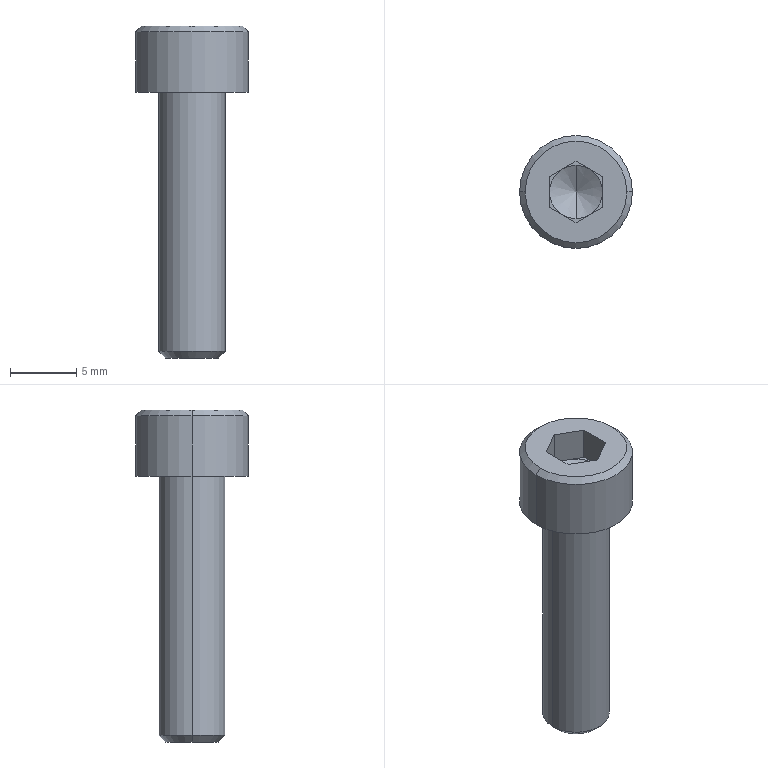Part | NX | features BREP 1 | 1 solid | 25 faces | box 8.5 x 8.5 x 25 mm | volume 632.849 mm3 | plane 15 | cone 6 | cylinder 4 | commonest cylinder face diameters 5 x2 8.5 x2
STEP:
#1=CARTESIAN_POINT('',(0.,-2.,2.5));
#2=VERTEX_POINT('',#1);
#3=CARTESIAN_POINT('',(0.,0.,1.345));
#4=VERTEX_POINT('',#3);
#5=CARTESIAN_POINT('',(0.,0.,1.345));
#6=DIRECTION('',(0.,-0.866,0.5));
#7=VECTOR('',#6,1000.);
#8=LINE('',#5,#7);
#9=EDGE_CURVE('',#2,#4,#8,.F.);
#10=ORIENTED_EDGE('',*,*,#9,.T.);
#11=CARTESIAN_POINT('',(0.,2.,2.5));
#12=VERTEX_POINT('',#11);
#13=CARTESIAN_POINT('',(0.,0.,1.345));
#14=DIRECTION('',(0.,0.866,0.5));
#15=VECTOR('',#14,1000.);
#16=LINE('',#13,#15);
#17=EDGE_CURVE('',#12,#4,#16,.F.);
#18=ORIENTED_EDGE('',*,*,#17,.F.);
#19=CARTESIAN_POINT('',(-1.,1.732,2.5));
#20=VERTEX_POINT('',#19);
#21=CARTESIAN_POINT('',(0.,0.,2.5));
#22=DIRECTION('',(0.,0.,1.));
#23=DIRECTION('',(0.,-1.,0.));
#24=AXIS2_PLACEMENT_3D('',#21,#22,#23);
#25=CIRCLE('',#24,2.);
#26=EDGE_CURVE('',#12,#20,#25,.T.);
#27=ORIENTED_EDGE('',*,*,#26,.T.);
#28=CARTESIAN_POINT('',(-2.,0.,2.5));
#29=VERTEX_POINT('',#28);
#30=CARTESIAN_POINT('',(0.,0.,2.5));
#31=DIRECTION('',(0.,0.,1.));
#32=DIRECTION('',(0.,-1.,0.));
#33=AXIS2_PLACEMENT_3D('',#30,#31,#32);
#34=CIRCLE('',#33,2.);
#35=EDGE_CURVE('',#20,#29,#34,.T.);
#36=ORIENTED_EDGE('',*,*,#35,.T.);
#37=CARTESIAN_POINT('',(-1.,-1.732,2.5));
#38=VERTEX_POINT('',#37);
#39=CARTESIAN_POINT('',(0.,0.,2.5));
#40=DIRECTION('',(0.,0.,1.));
#41=DIRECTION('',(0.,-1.,0.));
#42=AXIS2_PLACEMENT_3D('',#39,#40,#41);
#43=CIRCLE('',#42,2.);
#44=EDGE_CURVE('',#29,#38,#43,.T.);
#45=ORIENTED_EDGE('',*,*,#44,.T.);
#46=CARTESIAN_POINT('',(0.,0.,2.5));
#47=DIRECTION('',(0.,0.,1.));
#48=DIRECTION('',(0.,-1.,0.));
#49=AXIS2_PLACEMENT_3D('',#46,#47,#48);
#50=CIRCLE('',#49,2.);
#51=EDGE_CURVE('',#38,#2,#50,.T.);
#52=ORIENTED_EDGE('',*,*,#51,.T.);
#53=EDGE_LOOP('',(#10,#18,#27,#36,#45,#52));
#54=FACE_BOUND('',#53,.T.);
#55=CARTESIAN_POINT('',(0.,0.,1001.345));
#56=DIRECTION('',(0.,0.,1.));
#57=DIRECTION('',(0.,1.,0.));
#58=AXIS2_PLACEMENT_3D('',#55,#56,#57);
#59=CONICAL_SURFACE('',#58,1732.051,1.047);
#60=ADVANCED_FACE('',(#54),#59,.F.);
#61=CARTESIAN_POINT('',(4.25,0.,0.));
#62=VERTEX_POINT('',#61);
#63=CARTESIAN_POINT('',(-4.25,0.,0.));
#64=VERTEX_POINT('',#63);
#65=CARTESIAN_POINT('',(0.,0.,0.));
#66=DIRECTION('',(0.,0.,1.));
#67=DIRECTION('',(1.,0.,0.));
#68=AXIS2_PLACEMENT_3D('',#65,#66,#67);
#69=CIRCLE('',#68,4.25);
#70=EDGE_CURVE('',#62,#64,#69,.T.);
#71=ORIENTED_EDGE('',*,*,#70,.T.);
#72=CARTESIAN_POINT('',(-4.25,0.,4.575));
#73=VERTEX_POINT('',#72);
#74=CARTESIAN_POINT('',(-4.25,0.,0.));
#75=DIRECTION('',(0.,0.,1.));
#76=VECTOR('',#75,1000.);
#77=LINE('',#74,#76);
#78=EDGE_CURVE('',#64,#73,#77,.T.);
#79=ORIENTED_EDGE('',*,*,#78,.T.);
#80=CARTESIAN_POINT('',(4.25,0.,4.575));
#81=VERTEX_POINT('',#80);
#82=CARTESIAN_POINT('',(0.,0.,4.575));
#83=DIRECTION('',(0.,0.,1.));
#84=DIRECTION('',(1.,0.,0.));
#85=AXIS2_PLACEMENT_3D('',#82,#83,#84);
#86=CIRCLE('',#85,4.25);
#87=EDGE_CURVE('',#81,#73,#86,.T.);
#88=ORIENTED_EDGE('',*,*,#87,.F.);
#89=CARTESIAN_POINT('',(4.25,0.,0.));
#90=DIRECTION('',(0.,0.,1.));
#91=VECTOR('',#90,1000.);
#92=LINE('',#89,#91);
#93=EDGE_CURVE('',#62,#81,#92,.T.);
#94=ORIENTED_EDGE('',*,*,#93,.F.);
#95=EDGE_LOOP('',(#71,#79,#88,#94));
#96=FACE_BOUND('',#95,.T.);
#97=CARTESIAN_POINT('',(0.,0.,0.));
#98=DIRECTION('',(0.,0.,1.));
#99=DIRECTION('',(-1.,0.,0.));
#100=AXIS2_PLACEMENT_3D('',#97,#98,#99);
#101=CYLINDRICAL_SURFACE('',#100,4.25);
#102=ADVANCED_FACE('',(#96),#101,.T.);
#103=CARTESIAN_POINT('',(3.825,0.,5.));
#104=VERTEX_POINT('',#103);
#105=CARTESIAN_POINT('',(-3.825,0.,5.));
#106=VERTEX_POINT('',#105);
#107=CARTESIAN_POINT('',(0.,0.,5.));
#108=DIRECTION('',(0.,0.,1.));
#109=DIRECTION('',(1.,0.,0.));
#110=AXIS2_PLACEMENT_3D('',#107,#108,#109);
#111=CIRCLE('',#110,3.825);
#112=EDGE_CURVE('',#104,#106,#111,.T.);
#113=ORIENTED_EDGE('',*,*,#112,.F.);
#114=CARTESIAN_POINT('',(4.25,0.,4.575));
#115=DIRECTION('',(0.7071,0.,-0.7071));
#116=VECTOR('',#115,1000.);
#117=LINE('',#114,#116);
#118=EDGE_CURVE('',#81,#104,#117,.F.);
#119=ORIENTED_EDGE('',*,*,#118,.F.);
#120=ORIENTED_EDGE('',*,*,#87,.T.);
#121=CARTESIAN_POINT('',(-4.25,0.,4.575));
#122=DIRECTION('',(-0.7071,0.,-0.7071));
#123=VECTOR('',#122,1000.);
#124=LINE('',#121,#123);
#125=EDGE_CURVE('',#73,#106,#124,.F.);
#126=ORIENTED_EDGE('',*,*,#125,.T.);
#127=EDGE_LOOP('',(#113,#119,#120,#126));
#128=FACE_BOUND('',#127,.T.);
#129=CARTESIAN_POINT('',(0.,0.,4.575));
#130=DIRECTION('',(0.,0.,-1.));
#131=DIRECTION('',(1.,0.,0.));
#132=AXIS2_PLACEMENT_3D('',#129,#130,#131);
#133=CONICAL_SURFACE('',#132,4.25,0.7854);
#134=ADVANCED_FACE('',(#128),#133,.T.);
#135=CARTESIAN_POINT('',(2.01,0.,-20.));
#136=VERTEX_POINT('',#135);
#137=CARTESIAN_POINT('',(-2.01,0.,-20.));
#138=VERTEX_POINT('',#137);
#139=CARTESIAN_POINT('',(0.,0.,-20.));
#140=DIRECTION('',(0.,0.,1.));
#141=DIRECTION('',(1.,0.,0.));
#142=AXIS2_PLACEMENT_3D('',#139,#140,#141);
#143=CIRCLE('',#142,2.01);
#144=EDGE_CURVE('',#136,#138,#143,.T.);
#145=ORIENTED_EDGE('',*,*,#144,.T.);
#146=CARTESIAN_POINT('',(-2.5,0.,-19.509));
#147=VERTEX_POINT('',#146);
#148=CARTESIAN_POINT('',(-2.01,0.,-20.));
#149=DIRECTION('',(-0.7071,0.,0.7071));
#150=VECTOR('',#149,1000.);
#151=LINE('',#148,#150);
#152=EDGE_CURVE('',#138,#147,#151,.T.);
#153=ORIENTED_EDGE('',*,*,#152,.T.);
#154=CARTESIAN_POINT('',(2.5,0.,-19.509));
#155=VERTEX_POINT('',#154);
#156=CARTESIAN_POINT('',(0.,0.,-19.509));
#157=DIRECTION('',(0.,0.,1.));
#158=DIRECTION('',(1.,0.,0.));
#159=AXIS2_PLACEMENT_3D('',#156,#157,#158);
#160=CIRCLE('',#159,2.5);
#161=EDGE_CURVE('',#155,#147,#160,.T.);
#162=ORIENTED_EDGE('',*,*,#161,.F.);
#163=CARTESIAN_POINT('',(2.01,0.,-20.));
#164=DIRECTION('',(0.7071,0.,0.7071));
#165=VECTOR('',#164,1000.);
#166=LINE('',#163,#165);
#167=EDGE_CURVE('',#136,#155,#166,.T.);
#168=ORIENTED_EDGE('',*,*,#167,.F.);
#169=EDGE_LOOP('',(#145,#153,#162,#168));
#170=FACE_BOUND('',#169,.T.);
#171=CARTESIAN_POINT('',(0.,0.,-20.));
#172=DIRECTION('',(0.,0.,1.));
#173=DIRECTION('',(-1.,0.,0.));
#174=AXIS2_PLACEMENT_3D('',#171,#172,#173);
#175=CONICAL_SURFACE('',#174,2.01,0.7854);
#176=ADVANCED_FACE('',(#170),#175,.T.);
#177=ORIENTED_EDGE('',*,*,#161,.T.);
#178=CARTESIAN_POINT('',(-2.5,0.,0.));
#179=VERTEX_POINT('',#178);
#180=CARTESIAN_POINT('',(-2.5,0.,-20.));
#181=DIRECTION('',(0.,0.,1.));
#182=VECTOR('',#181,1000.);
#183=LINE('',#180,#182);
#184=EDGE_CURVE('',#147,#179,#183,.T.);
#185=ORIENTED_EDGE('',*,*,#184,.T.);
#186=CARTESIAN_POINT('',(2.5,0.,0.));
#187=VERTEX_POINT('',#186);
#188=CARTESIAN_POINT('',(0.,0.,0.));
#189=DIRECTION('',(0.,0.,1.));
#190=DIRECTION('',(1.,0.,0.));
#191=AXIS2_PLACEMENT_3D('',#188,#189,#190);
#192=CIRCLE('',#191,2.5);
#193=EDGE_CURVE('',#187,#179,#192,.T.);
#194=ORIENTED_EDGE('',*,*,#193,.F.);
#195=CARTESIAN_POINT('',(2.5,0.,-20.));
#196=DIRECTION('',(0.,0.,1.));
#197=VECTOR('',#196,1000.);
#198=LINE('',#195,#197);
#199=EDGE_CURVE('',#155,#187,#198,.T.);
#200=ORIENTED_EDGE('',*,*,#199,.F.);
#201=EDGE_LOOP('',(#177,#185,#194,#200));
#202=FACE_BOUND('',#201,.T.);
#203=CARTESIAN_POINT('',(0.,0.,-20.));
#204=DIRECTION('',(0.,0.,1.));
#205=DIRECTION('',(-1.,0.,0.));
#206=AXIS2_PLACEMENT_3D('',#203,#204,#205);
#207=CYLINDRICAL_SURFACE('',#206,2.5);
#208=ADVANCED_FACE('',(#202),#207,.T.);
#209=CARTESIAN_POINT('',(1.,-1.732,2.5));
#210=VERTEX_POINT('',#209);
#211=CARTESIAN_POINT('',(2.,0.,2.5));
#212=VERTEX_POINT('',#211);
#213=CARTESIAN_POINT('',(0.,0.,2.5));
#214=DIRECTION('',(0.,0.,1.));
#215=DIRECTION('',(0.,-1.,0.));
#216=AXIS2_PLACEMENT_3D('',#213,#214,#215);
#217=CIRCLE('',#216,2.);
#218=EDGE_CURVE('',#210,#212,#217,.T.);
#219=ORIENTED_EDGE('',*,*,#218,.F.);
#220=CARTESIAN_POINT('',(2.,-1.155,2.5));
#221=VERTEX_POINT('',#220);
#222=CARTESIAN_POINT('',(0.,-2.309,2.5));
#223=DIRECTION('',(0.866,0.5,0.));
#224=VECTOR('',#223,1000.);
#225=LINE('',#222,#224);
#226=EDGE_CURVE('',#210,#221,#225,.T.);
#227=ORIENTED_EDGE('',*,*,#226,.T.);
#228=CARTESIAN_POINT('',(2.,-1.155,2.5));
#229=DIRECTION('',(0.,1.,0.));
#230=VECTOR('',#229,1000.);
#231=LINE('',#228,#230);
#232=EDGE_CURVE('',#221,#212,#231,.T.);
#233=ORIENTED_EDGE('',*,*,#232,.T.);
#234=EDGE_LOOP('',(#219,#227,#233));
#235=FACE_BOUND('',#234,.T.);
#236=CARTESIAN_POINT('',(0.,0.,2.5));
#237=DIRECTION('',(0.,0.,1.));
#238=DIRECTION('',(-1.,0.,0.));
#239=AXIS2_PLACEMENT_3D('',#236,#237,#238);
#240=PLANE('',#239);
#241=ADVANCED_FACE('',(#235),#240,.T.);
#242=CARTESIAN_POINT('',(1.,1.732,2.5));
#243=VERTEX_POINT('',#242);
#244=CARTESIAN_POINT('',(0.,0.,2.5));
#245=DIRECTION('',(0.,0.,1.));
#246=DIRECTION('',(0.,-1.,0.));
#247=AXIS2_PLACEMENT_3D('',#244,#245,#246);
#248=CIRCLE('',#247,2.);
#249=EDGE_CURVE('',#212,#243,#248,.T.);
#250=ORIENTED_EDGE('',*,*,#249,.F.);
#251=CARTESIAN_POINT('',(2.,1.155,2.5));
#252=VERTEX_POINT('',#251);
#253=CARTESIAN_POINT('',(2.,-1.155,2.5));
#254=DIRECTION('',(0.,1.,0.));
#255=VECTOR('',#254,1000.);
#256=LINE('',#253,#255);
#257=EDGE_CURVE('',#212,#252,#256,.T.);
#258=ORIENTED_EDGE('',*,*,#257,.T.);
#259=CARTESIAN_POINT('',(2.,1.155,2.5));
#260=DIRECTION('',(-0.866,0.5,0.));
#261=VECTOR('',#260,1000.);
#262=LINE('',#259,#261);
#263=EDGE_CURVE('',#252,#243,#262,.T.);
#264=ORIENTED_EDGE('',*,*,#263,.T.);
#265=EDGE_LOOP('',(#250,#258,#264));
#266=FACE_BOUND('',#265,.T.);
#267=CARTESIAN_POINT('',(0.,0.,2.5));
#268=DIRECTION('',(0.,0.,1.));
#269=DIRECTION('',(-1.,0.,0.));
#270=AXIS2_PLACEMENT_3D('',#267,#268,#269);
#271=PLANE('',#270);
#272=ADVANCED_FACE('',(#266),#271,.T.);
#273=CARTESIAN_POINT('',(0.,0.,2.5));
#274=DIRECTION('',(0.,0.,1.));
#275=DIRECTION('',(0.,-1.,0.));
#276=AXIS2_PLACEMENT_3D('',#273,#274,#275);
#277=CIRCLE('',#276,2.);
#278=EDGE_CURVE('',#243,#12,#277,.T.);
#279=ORIENTED_EDGE('',*,*,#278,.F.);
#280=CARTESIAN_POINT('',(0.,2.309,2.5));
#281=VERTEX_POINT('',#280);
#282=CARTESIAN_POINT('',(2.,1.155,2.5));
#283=DIRECTION('',(-0.866,0.5,0.));
#284=VECTOR('',#283,1000.);
#285=LINE('',#282,#284);
#286=EDGE_CURVE('',#243,#281,#285,.T.);
#287=ORIENTED_EDGE('',*,*,#286,.T.);
#288=CARTESIAN_POINT('',(0.,2.309,2.5));
#289=DIRECTION('',(-0.866,-0.5,0.));
#290=VECTOR('',#289,1000.);
#291=LINE('',#288,#290);
#292=EDGE_CURVE('',#281,#20,#291,.T.);
#293=ORIENTED_EDGE('',*,*,#292,.T.);
#294=ORIENTED_EDGE('',*,*,#26,.F.);
#295=EDGE_LOOP('',(#279,#287,#293,#294));
#296=FACE_BOUND('',#295,.T.);
#297=CARTESIAN_POINT('',(0.,0.,2.5));
#298=DIRECTION('',(0.,0.,1.));
#299=DIRECTION('',(-1.,0.,0.));
#300=AXIS2_PLACEMENT_3D('',#297,#298,#299);
#301=PLANE('',#300);
#302=ADVANCED_FACE('',(#296),#301,.T.);
#303=ORIENTED_EDGE('',*,*,#35,.F.);
#304=CARTESIAN_POINT('',(-2.,1.155,2.5));
#305=VERTEX_POINT('',#304);
#306=CARTESIAN_POINT('',(0.,2.309,2.5));
#307=DIRECTION('',(-0.866,-0.5,0.));
#308=VECTOR('',#307,1000.);
#309=LINE('',#306,#308);
#310=EDGE_CURVE('',#20,#305,#309,.T.);
#311=ORIENTED_EDGE('',*,*,#310,.T.);
#312=CARTESIAN_POINT('',(-2.,1.155,2.5));
#313=DIRECTION('',(0.,-1.,0.));
#314=VECTOR('',#313,1000.);
#315=LINE('',#312,#314);
#316=EDGE_CURVE('',#305,#29,#315,.T.);
#317=ORIENTED_EDGE('',*,*,#316,.T.);
#318=EDGE_LOOP('',(#303,#311,#317));
#319=FACE_BOUND('',#318,.T.);
#320=CARTESIAN_POINT('',(0.,0.,2.5));
#321=DIRECTION('',(0.,0.,1.));
#322=DIRECTION('',(-1.,0.,0.));
#323=AXIS2_PLACEMENT_3D('',#320,#321,#322);
#324=PLANE('',#323);
#325=ADVANCED_FACE('',(#319),#324,.T.);
#326=ORIENTED_EDGE('',*,*,#44,.F.);
#327=CARTESIAN_POINT('',(-2.,-1.155,2.5));
#328=VERTEX_POINT('',#327);
#329=CARTESIAN_POINT('',(-2.,1.155,2.5));
#330=DIRECTION('',(0.,-1.,0.));
#331=VECTOR('',#330,1000.);
#332=LINE('',#329,#331);
#333=EDGE_CURVE('',#29,#328,#332,.T.);
#334=ORIENTED_EDGE('',*,*,#333,.T.);
#335=CARTESIAN_POINT('',(-2.,-1.155,2.5));
#336=DIRECTION('',(0.866,-0.5,0.));
#337=VECTOR('',#336,1000.);
#338=LINE('',#335,#337);
#339=EDGE_CURVE('',#328,#38,#338,.T.);
#340=ORIENTED_EDGE('',*,*,#339,.T.);
#341=EDGE_LOOP('',(#326,#334,#340));
#342=FACE_BOUND('',#341,.T.);
#343=CARTESIAN_POINT('',(0.,0.,2.5));
#344=DIRECTION('',(0.,0.,1.));
#345=DIRECTION('',(-1.,0.,0.));
#346=AXIS2_PLACEMENT_3D('',#343,#344,#345);
#347=PLANE('',#346);
#348=ADVANCED_FACE('',(#342),#347,.T.);
#349=ORIENTED_EDGE('',*,*,#184,.F.);
#350=CARTESIAN_POINT('',(0.,0.,-19.509));
#351=DIRECTION('',(0.,0.,1.));
#352=DIRECTION('',(1.,0.,0.));
#353=AXIS2_PLACEMENT_3D('',#350,#351,#352);
#354=CIRCLE('',#353,2.5);
#355=EDGE_CURVE('',#147,#155,#354,.T.);
#356=ORIENTED_EDGE('',*,*,#355,.T.);
#357=ORIENTED_EDGE('',*,*,#199,.T.);
#358=CARTESIAN_POINT('',(0.,0.,0.));
#359=DIRECTION('',(0.,0.,1.));
#360=DIRECTION('',(1.,0.,0.));
#361=AXIS2_PLACEMENT_3D('',#358,#359,#360);
#362=CIRCLE('',#361,2.5);
#363=EDGE_CURVE('',#179,#187,#362,.T.);
#364=ORIENTED_EDGE('',*,*,#363,.F.);
#365=EDGE_LOOP('',(#349,#356,#357,#364));
#366=FACE_BOUND('',#365,.T.);
#367=CARTESIAN_POINT('',(0.,0.,-20.));
#368=DIRECTION('',(0.,0.,1.));
#369=DIRECTION('',(-1.,0.,0.));
#370=AXIS2_PLACEMENT_3D('',#367,#368,#369);
#371=CYLINDRICAL_SURFACE('',#370,2.5);
#372=ADVANCED_FACE('',(#366),#371,.T.);
#373=ORIENTED_EDGE('',*,*,#152,.F.);
#374=CARTESIAN_POINT('',(0.,0.,-20.));
#375=DIRECTION('',(0.,0.,1.));
#376=DIRECTION('',(1.,0.,0.));
#377=AXIS2_PLACEMENT_3D('',#374,#375,#376);
#378=CIRCLE('',#377,2.01);
#379=EDGE_CURVE('',#138,#136,#378,.T.);
#380=ORIENTED_EDGE('',*,*,#379,.T.);
#381=ORIENTED_EDGE('',*,*,#167,.T.);
#382=ORIENTED_EDGE('',*,*,#355,.F.);
#383=EDGE_LOOP('',(#373,#380,#381,#382));
#384=FACE_BOUND('',#383,.T.);
#385=CARTESIAN_POINT('',(0.,0.,-20.));
#386=DIRECTION('',(0.,0.,1.));
#387=DIRECTION('',(-1.,0.,0.));
#388=AXIS2_PLACEMENT_3D('',#385,#386,#387);
#389=CONICAL_SURFACE('',#388,2.01,0.7854);
#390=ADVANCED_FACE('',(#384),#389,.T.);
#391=ORIENTED_EDGE('',*,*,#144,.F.);
#392=ORIENTED_EDGE('',*,*,#379,.F.);
#393=EDGE_LOOP('',(#391,#392));
#394=FACE_BOUND('',#393,.T.);
#395=CARTESIAN_POINT('',(0.,2.01,-20.));
#396=DIRECTION('',(0.,0.,1.));
#397=DIRECTION('',(-1.,0.,0.));
#398=AXIS2_PLACEMENT_3D('',#395,#396,#397);
#399=PLANE('',#398);
#400=ADVANCED_FACE('',(#394),#399,.F.);
#401=CARTESIAN_POINT('',(0.,-2.309,5.));
#402=VERTEX_POINT('',#401);
#403=CARTESIAN_POINT('',(2.,-1.155,5.));
#404=VERTEX_POINT('',#403);
#405=CARTESIAN_POINT('',(0.,-2.309,5.));
#406=DIRECTION('',(0.866,0.5,0.));
#407=VECTOR('',#406,1000.);
#408=LINE('',#405,#407);
#409=EDGE_CURVE('',#402,#404,#408,.T.);
#410=ORIENTED_EDGE('',*,*,#409,.F.);
#411=CARTESIAN_POINT('',(-2.,-1.155,5.));
#412=VERTEX_POINT('',#411);
#413=CARTESIAN_POINT('',(-2.,-1.155,5.));
#414=DIRECTION('',(0.866,-0.5,0.));
#415=VECTOR('',#414,1000.);
#416=LINE('',#413,#415);
#417=EDGE_CURVE('',#412,#402,#416,.T.);
#418=ORIENTED_EDGE('',*,*,#417,.F.);
#419=CARTESIAN_POINT('',(-2.,1.155,5.));
#420=VERTEX_POINT('',#419);
#421=CARTESIAN_POINT('',(-2.,1.155,5.));
#422=DIRECTION('',(0.,-1.,0.));
#423=VECTOR('',#422,1000.);
#424=LINE('',#421,#423);
#425=EDGE_CURVE('',#420,#412,#424,.T.);
#426=ORIENTED_EDGE('',*,*,#425,.F.);
#427=CARTESIAN_POINT('',(0.,2.309,5.));
#428=VERTEX_POINT('',#427);
#429=CARTESIAN_POINT('',(0.,2.309,5.));
#430=DIRECTION('',(-0.866,-0.5,0.));
#431=VECTOR('',#430,1000.);
#432=LINE('',#429,#431);
#433=EDGE_CURVE('',#428,#420,#432,.T.);
#434=ORIENTED_EDGE('',*,*,#433,.F.);
#435=CARTESIAN_POINT('',(2.,1.155,5.));
#436=VERTEX_POINT('',#435);
#437=CARTESIAN_POINT('',(2.,1.155,5.));
#438=DIRECTION('',(-0.866,0.5,0.));
#439=VECTOR('',#438,1000.);
#440=LINE('',#437,#439);
#441=EDGE_CURVE('',#436,#428,#440,.T.);
#442=ORIENTED_EDGE('',*,*,#441,.F.);
#443=CARTESIAN_POINT('',(2.,-1.155,5.));
#444=DIRECTION('',(0.,1.,0.));
#445=VECTOR('',#444,1000.);
#446=LINE('',#443,#445);
#447=EDGE_CURVE('',#404,#436,#446,.T.);
#448=ORIENTED_EDGE('',*,*,#447,.F.);
#449=EDGE_LOOP('',(#410,#418,#426,#434,#442,#448));
#450=FACE_BOUND('',#449,.T.);
#451=CARTESIAN_POINT('',(0.,0.,5.));
#452=DIRECTION('',(0.,0.,1.));
#453=DIRECTION('',(1.,0.,0.));
#454=AXIS2_PLACEMENT_3D('',#451,#452,#453);
#455=CIRCLE('',#454,3.825);
#456=EDGE_CURVE('',#106,#104,#455,.T.);
#457=ORIENTED_EDGE('',*,*,#456,.T.);
#458=ORIENTED_EDGE('',*,*,#112,.T.);
#459=EDGE_LOOP('',(#457,#458));
#460=FACE_BOUND('',#459,.T.);
#461=CARTESIAN_POINT('',(0.,0.,5.));
#462=DIRECTION('',(0.,0.,-1.));
#463=DIRECTION('',(1.,0.,0.));
#464=AXIS2_PLACEMENT_3D('',#461,#462,#463);
#465=PLANE('',#464);
#466=ADVANCED_FACE('',(#450,#460),#465,.F.);
#467=ORIENTED_EDGE('',*,*,#118,.T.);
#468=ORIENTED_EDGE('',*,*,#456,.F.);
#469=ORIENTED_EDGE('',*,*,#125,.F.);
#470=CARTESIAN_POINT('',(0.,0.,4.575));
#471=DIRECTION('',(0.,0.,1.));
#472=DIRECTION('',(1.,0.,0.));
#473=AXIS2_PLACEMENT_3D('',#470,#471,#472);
#474=CIRCLE('',#473,4.25);
#475=EDGE_CURVE('',#73,#81,#474,.T.);
#476=ORIENTED_EDGE('',*,*,#475,.T.);
#477=EDGE_LOOP('',(#467,#468,#469,#476));
#478=FACE_BOUND('',#477,.T.);
#479=CARTESIAN_POINT('',(0.,0.,4.575));
#480=DIRECTION('',(0.,0.,-1.));
#481=DIRECTION('',(1.,0.,0.));
#482=AXIS2_PLACEMENT_3D('',#479,#480,#481);
#483=CONICAL_SURFACE('',#482,4.25,0.7854);
#484=ADVANCED_FACE('',(#478),#483,.T.);
#485=ORIENTED_EDGE('',*,*,#78,.F.);
#486=CARTESIAN_POINT('',(0.,0.,0.));
#487=DIRECTION('',(0.,0.,1.));
#488=DIRECTION('',(1.,0.,0.));
#489=AXIS2_PLACEMENT_3D('',#486,#487,#488);
#490=CIRCLE('',#489,4.25);
#491=EDGE_CURVE('',#64,#62,#490,.T.);
#492=ORIENTED_EDGE('',*,*,#491,.T.);
#493=ORIENTED_EDGE('',*,*,#93,.T.);
#494=ORIENTED_EDGE('',*,*,#475,.F.);
#495=EDGE_LOOP('',(#485,#492,#493,#494));
#496=FACE_BOUND('',#495,.T.);
#497=CARTESIAN_POINT('',(0.,0.,0.));
#498=DIRECTION('',(0.,0.,1.));
#499=DIRECTION('',(-1.,0.,0.));
#500=AXIS2_PLACEMENT_3D('',#497,#498,#499);
#501=CYLINDRICAL_SURFACE('',#500,4.25);
#502=ADVANCED_FACE('',(#496),#501,.T.);
#503=ORIENTED_EDGE('',*,*,#193,.T.);
#504=ORIENTED_EDGE('',*,*,#363,.T.);
#505=EDGE_LOOP('',(#503,#504));
#506=FACE_BOUND('',#505,.T.);
#507=ORIENTED_EDGE('',*,*,#70,.F.);
#508=ORIENTED_EDGE('',*,*,#491,.F.);
#509=EDGE_LOOP('',(#507,#508));
#510=FACE_BOUND('',#509,.T.);
#511=CARTESIAN_POINT('',(0.,4.25,0.));
#512=DIRECTION('',(0.,0.,1.));
#513=DIRECTION('',(-1.,0.,0.));
#514=AXIS2_PLACEMENT_3D('',#511,#512,#513);
#515=PLANE('',#514);
#516=ADVANCED_FACE('',(#506,#510),#515,.F.);
#517=ORIENTED_EDGE('',*,*,#417,.T.);
#518=CARTESIAN_POINT('',(0.,-2.309,2.5));
#519=VERTEX_POINT('',#518);
#520=CARTESIAN_POINT('',(0.,-2.309,2.5));
#521=DIRECTION('',(0.,0.,1.));
#522=VECTOR('',#521,1000.);
#523=LINE('',#520,#522);
#524=EDGE_CURVE('',#519,#402,#523,.T.);
#525=ORIENTED_EDGE('',*,*,#524,.F.);
#526=CARTESIAN_POINT('',(-2.,-1.155,2.5));
#527=DIRECTION('',(0.866,-0.5,0.));
#528=VECTOR('',#527,1000.);
#529=LINE('',#526,#528);
#530=EDGE_CURVE('',#38,#519,#529,.T.);
#531=ORIENTED_EDGE('',*,*,#530,.F.);
#532=ORIENTED_EDGE('',*,*,#339,.F.);
#533=CARTESIAN_POINT('',(-2.,-1.155,2.5));
#534=DIRECTION('',(0.,0.,1.));
#535=VECTOR('',#534,1000.);
#536=LINE('',#533,#535);
#537=EDGE_CURVE('',#328,#412,#536,.T.);
#538=ORIENTED_EDGE('',*,*,#537,.T.);
#539=EDGE_LOOP('',(#517,#525,#531,#532,#538));
#540=FACE_BOUND('',#539,.T.);
#541=CARTESIAN_POINT('',(-2.,-1.155,2.5));
#542=DIRECTION('',(-0.5,-0.866,0.));
#543=DIRECTION('',(-0.866,0.5,0.));
#544=AXIS2_PLACEMENT_3D('',#541,#542,#543);
#545=PLANE('',#544);
#546=ADVANCED_FACE('',(#540),#545,.F.);
#547=ORIENTED_EDGE('',*,*,#425,.T.);
#548=ORIENTED_EDGE('',*,*,#537,.F.);
#549=ORIENTED_EDGE('',*,*,#333,.F.);
#550=ORIENTED_EDGE('',*,*,#316,.F.);
#551=CARTESIAN_POINT('',(-2.,1.155,2.5));
#552=DIRECTION('',(0.,0.,1.));
#553=VECTOR('',#552,1000.);
#554=LINE('',#551,#553);
#555=EDGE_CURVE('',#305,#420,#554,.T.);
#556=ORIENTED_EDGE('',*,*,#555,.T.);
#557=EDGE_LOOP('',(#547,#548,#549,#550,#556));
#558=FACE_BOUND('',#557,.T.);
#559=CARTESIAN_POINT('',(-2.,1.155,2.5));
#560=DIRECTION('',(-1.,0.,0.));
#561=DIRECTION('',(0.,0.,-1.));
#562=AXIS2_PLACEMENT_3D('',#559,#560,#561);
#563=PLANE('',#562);
#564=ADVANCED_FACE('',(#558),#563,.F.);
#565=ORIENTED_EDGE('',*,*,#433,.T.);
#566=ORIENTED_EDGE('',*,*,#555,.F.);
#567=ORIENTED_EDGE('',*,*,#310,.F.);
#568=ORIENTED_EDGE('',*,*,#292,.F.);
#569=CARTESIAN_POINT('',(0.,2.309,2.5));
#570=DIRECTION('',(0.,0.,1.));
#571=VECTOR('',#570,1000.);
#572=LINE('',#569,#571);
#573=EDGE_CURVE('',#281,#428,#572,.T.);
#574=ORIENTED_EDGE('',*,*,#573,.T.);
#575=EDGE_LOOP('',(#565,#566,#567,#568,#574));
#576=FACE_BOUND('',#575,.T.);
#577=CARTESIAN_POINT('',(0.,2.309,2.5));
#578=DIRECTION('',(-0.5,0.866,0.));
#579=DIRECTION('',(0.866,0.5,0.));
#580=AXIS2_PLACEMENT_3D('',#577,#578,#579);
#581=PLANE('',#580);
#582=ADVANCED_FACE('',(#576),#581,.F.);
#583=ORIENTED_EDGE('',*,*,#441,.T.);
#584=ORIENTED_EDGE('',*,*,#573,.F.);
#585=ORIENTED_EDGE('',*,*,#286,.F.);
#586=ORIENTED_EDGE('',*,*,#263,.F.);
#587=CARTESIAN_POINT('',(2.,1.155,2.5));
#588=DIRECTION('',(0.,0.,1.));
#589=VECTOR('',#588,1000.);
#590=LINE('',#587,#589);
#591=EDGE_CURVE('',#252,#436,#590,.T.);
#592=ORIENTED_EDGE('',*,*,#591,.T.);
#593=EDGE_LOOP('',(#583,#584,#585,#586,#592));
#594=FACE_BOUND('',#593,.T.);
#595=CARTESIAN_POINT('',(2.,1.155,2.5));
#596=DIRECTION('',(0.5,0.866,0.));
#597=DIRECTION('',(0.866,-0.5,0.));
#598=AXIS2_PLACEMENT_3D('',#595,#596,#597);
#599=PLANE('',#598);
#600=ADVANCED_FACE('',(#594),#599,.F.);
#601=ORIENTED_EDGE('',*,*,#447,.T.);
#602=ORIENTED_EDGE('',*,*,#591,.F.);
#603=ORIENTED_EDGE('',*,*,#257,.F.);
#604=ORIENTED_EDGE('',*,*,#232,.F.);
#605=CARTESIAN_POINT('',(2.,-1.155,2.5));
#606=DIRECTION('',(0.,0.,1.));
#607=VECTOR('',#606,1000.);
#608=LINE('',#605,#607);
#609=EDGE_CURVE('',#221,#404,#608,.T.);
#610=ORIENTED_EDGE('',*,*,#609,.T.);
#611=EDGE_LOOP('',(#601,#602,#603,#604,#610));
#612=FACE_BOUND('',#611,.T.);
#613=CARTESIAN_POINT('',(2.,-1.155,2.5));
#614=DIRECTION('',(1.,0.,0.));
#615=DIRECTION('',(0.,0.,1.));
#616=AXIS2_PLACEMENT_3D('',#613,#614,#615);
#617=PLANE('',#616);
#618=ADVANCED_FACE('',(#612),#617,.F.);
#619=ORIENTED_EDGE('',*,*,#409,.T.);
#620=ORIENTED_EDGE('',*,*,#609,.F.);
#621=ORIENTED_EDGE('',*,*,#226,.F.);
#622=CARTESIAN_POINT('',(0.,-2.309,2.5));
#623=DIRECTION('',(0.866,0.5,0.));
#624=VECTOR('',#623,1000.);
#625=LINE('',#622,#624);
#626=EDGE_CURVE('',#519,#210,#625,.T.);
#627=ORIENTED_EDGE('',*,*,#626,.F.);
#628=ORIENTED_EDGE('',*,*,#524,.T.);
#629=EDGE_LOOP('',(#619,#620,#621,#627,#628));
#630=FACE_BOUND('',#629,.T.);
#631=CARTESIAN_POINT('',(0.,-2.309,2.5));
#632=DIRECTION('',(0.5,-0.866,0.));
#633=DIRECTION('',(-0.866,-0.5,0.));
#634=AXIS2_PLACEMENT_3D('',#631,#632,#633);
#635=PLANE('',#634);
#636=ADVANCED_FACE('',(#630),#635,.F.);
#637=ORIENTED_EDGE('',*,*,#51,.F.);
#638=ORIENTED_EDGE('',*,*,#530,.T.);
#639=ORIENTED_EDGE('',*,*,#626,.T.);
#640=CARTESIAN_POINT('',(0.,0.,2.5));
#641=DIRECTION('',(0.,0.,1.));
#642=DIRECTION('',(0.,-1.,0.));
#643=AXIS2_PLACEMENT_3D('',#640,#641,#642);
#644=CIRCLE('',#643,2.);
#645=EDGE_CURVE('',#2,#210,#644,.T.);
#646=ORIENTED_EDGE('',*,*,#645,.F.);
#647=EDGE_LOOP('',(#637,#638,#639,#646));
#648=FACE_BOUND('',#647,.T.);
#649=CARTESIAN_POINT('',(0.,0.,2.5));
#650=DIRECTION('',(0.,0.,1.));
#651=DIRECTION('',(-1.,0.,0.));
#652=AXIS2_PLACEMENT_3D('',#649,#650,#651);
#653=PLANE('',#652);
#654=ADVANCED_FACE('',(#648),#653,.T.);
#655=ORIENTED_EDGE('',*,*,#17,.T.);
#656=ORIENTED_EDGE('',*,*,#9,.F.);
#657=ORIENTED_EDGE('',*,*,#645,.T.);
#658=ORIENTED_EDGE('',*,*,#218,.T.);
#659=ORIENTED_EDGE('',*,*,#249,.T.);
#660=ORIENTED_EDGE('',*,*,#278,.T.);
#661=EDGE_LOOP('',(#655,#656,#657,#658,#659,#660));
#662=FACE_BOUND('',#661,.T.);
#663=CARTESIAN_POINT('',(0.,0.,1001.345));
#664=DIRECTION('',(0.,0.,1.));
#665=DIRECTION('',(0.,1.,0.));
#666=AXIS2_PLACEMENT_3D('',#663,#664,#665);
#667=CONICAL_SURFACE('',#666,1732.051,1.047);
#668=ADVANCED_FACE('',(#662),#667,.F.);
#669=CLOSED_SHELL('',(#60,#102,#134,#176,#208,#241,#272,#302,#325,#348,#372,#390,#400,#466,#484,#502,#516,#546,#564,#582,#600,#618,#636,#654,#668));
#670=MANIFOLD_SOLID_BREP('',#669);
#671=(LENGTH_UNIT()NAMED_UNIT(*)SI_UNIT(.MILLI.,.METRE.));
#672=UNCERTAINTY_MEASURE_WITH_UNIT(LENGTH_MEASURE(0.00001),#671,'','');
#673=(NAMED_UNIT(*)PLANE_ANGLE_UNIT()SI_UNIT($,.RADIAN.));
#674=(NAMED_UNIT(*)SI_UNIT($,.STERADIAN.)SOLID_ANGLE_UNIT());
#675=(GEOMETRIC_REPRESENTATION_CONTEXT(3)GLOBAL_UNCERTAINTY_ASSIGNED_CONTEXT((#672))GLOBAL_UNIT_ASSIGNED_CONTEXT((#671,#673,#674))REPRESENTATION_CONTEXT('',''));
#676=ADVANCED_BREP_SHAPE_REPRESENTATION('',(#670),#675);